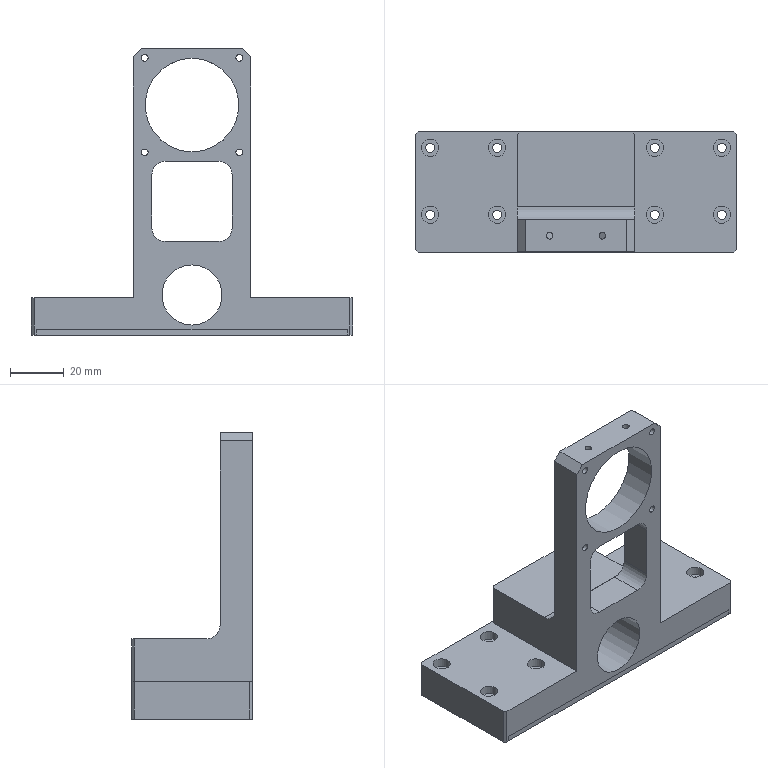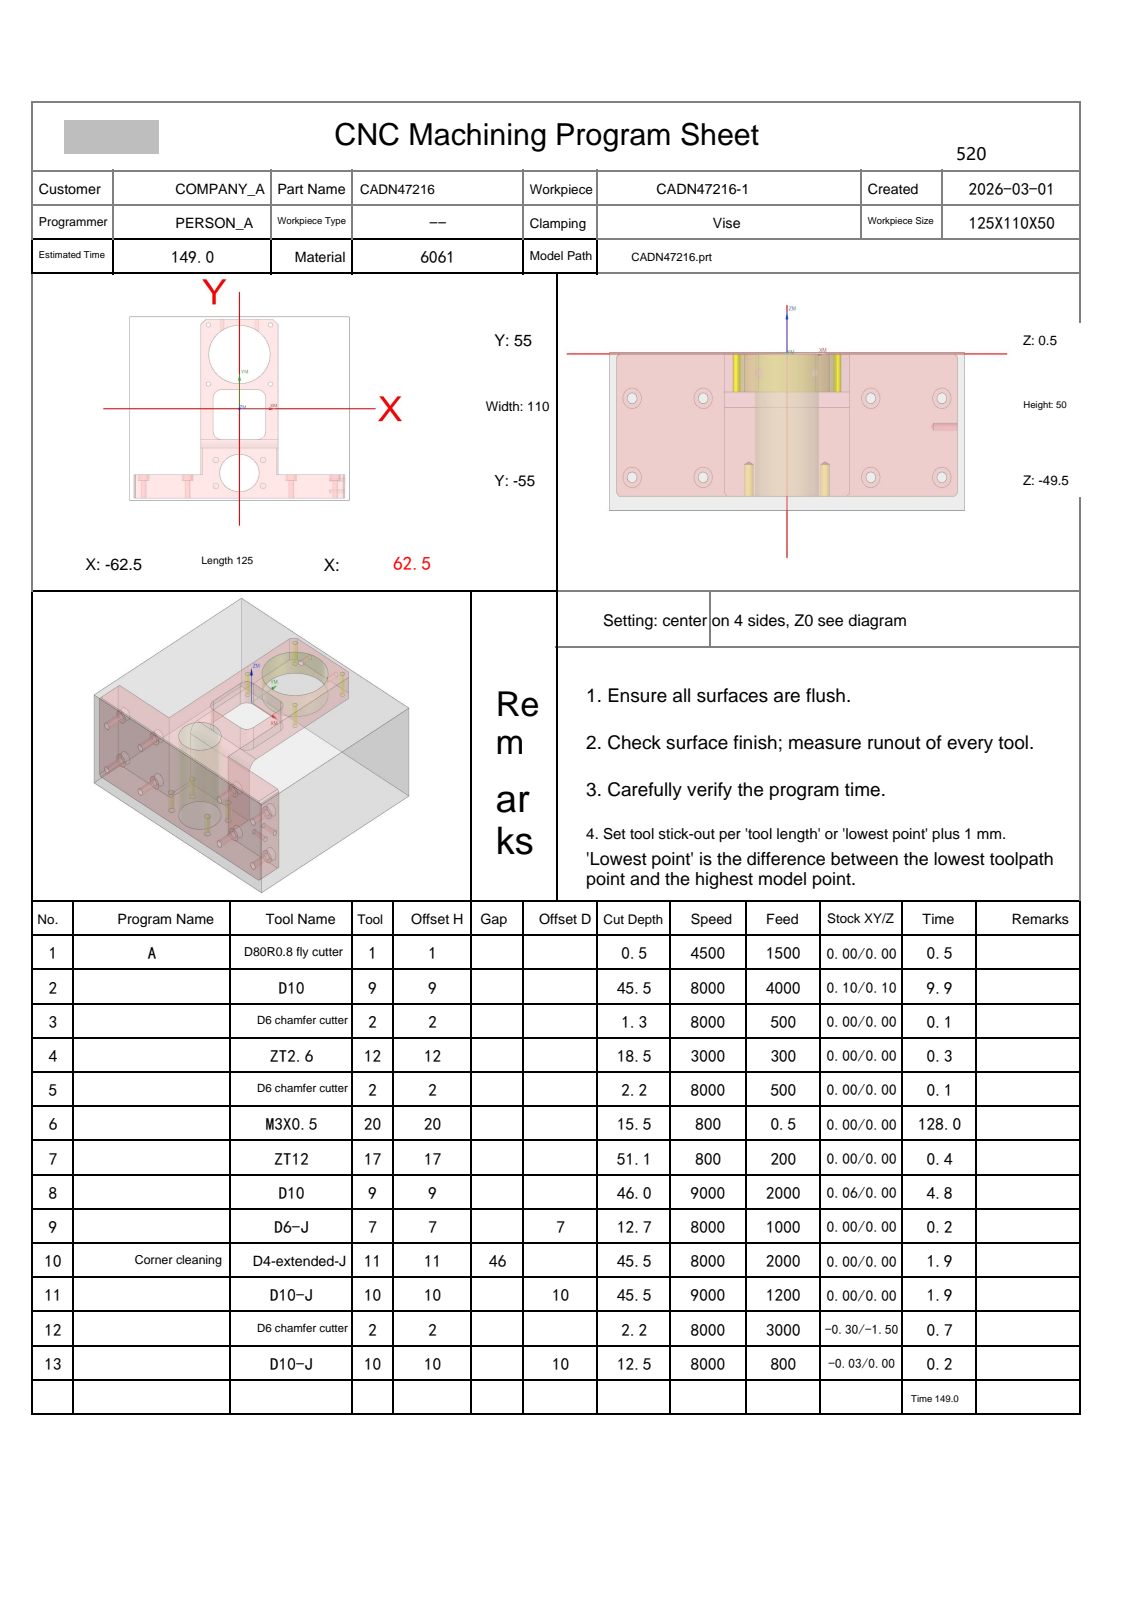NC program | NX | posted by the shop | part box 120 x 45 x 107 mm
Lines 6042 to 6508 of 16292:
N3 T02 M06
(D6 chamfer cutter  D=6. R=0. H=02 ce=0.00 di=0.10)
G00 G90 G54 X-17.678 Y50.178 M03 S8000
G43 H02 Z50.
M08
G98 G81 X-17.678 Y50.178 Z-.8 R1. F500.
X17.678
Y14.822
X0.0 Y32.5
X-17.678 Y14.822
X0.0 Y-38.5
G80
G00 Z50.
G91 G28 Z0.0
M05
M09
G91 G28 Z0.0
M01
N4 T12 M06
(ZT2.6 D=2.6 DR_a=118 H=12)
G00 G90 G54 X-17.678 Y50.178 M03 S3000
G43 H12 Z50.
M08
G98 G83 X-17.678 Y50.178 Z-18. R1. F300. Q2.
Y14.822
X17.678
Y50.178
G80
G00 Z50.
G91 G28 Z0.0
M05
M09
G91 G28 Z0.0
M01
N5 T02 M06
(D6 chamfer cutter  D=6. R=0. H=02 ce=0.00 di=0.10)
G00 G90 G54 X-17.678 Y50.178 M03 S8000
G43 H02 Z50.
M08
G98 G81 X-17.678 Y50.178 Z-1.75 R3. F500.
Y14.822
X17.678
Y50.178
G80
G00 Z50.
G91 G28 Z0.0
M05
M09
G91 G28 Z0.0
M01
N6 T20 M06
(M3X0.5 D=2.5 DR_a=180 H=20)
G00 G90 G54 X-17.678 Y50.178 M03 S800
G43 H20 Z50.
M08
G95
G98 G84 X-17.678 Y50.178 Z-15. R1. F.5 Q5.
Y14.822
X17.678
Y50.178
G80
G94
G00 Z50.
G91 G28 Z0.0
M05
M09
G91 G28 Z0.0
M01
N7 T17 M06
(ZT12 D=12. DR_a=118 H=17)
G00 G90 G54 X0.0 Y-38.5 M03 S800
G43 H17 Z50.
M08
G98 G83 X0.0 Y-38.5 Z-50.605 R1. F200. Q3.
G80
G00 Z50.
G00 G90 X0.0 Y32.5 M03 S800
Z50.
G98 G83 X0.0 Y32.5 Z-17.105 R1. F200. Q2.
G80
G00 Z50.
G91 G28 Z0.0
M05
M09
G91 G28 Z0.0
M01
N8 T09 M06
(D10  D=10. R=0. H=09 ce=0.10 di=0.00)
G00 G90 G54 X0.0 Y-13.4 M03 S9000
G43 H09 Z50.
M08
Z.5
G01 X9.9 Z.44 F2000.
Y6.4 Z.319
X-9.9 Z.199
Y-13.4 Z.079
X9.9 Z-.042
Y6.4 Z-.162
X-9.9 Z-.282
Y-13.4 Z-.403
X9.9 Z-.523
Y6.4 Z-.644
X-9.9 Z-.764
Y-13.4 Z-.884
X9.9 Z-1.005
Y6.4 Z-1.125
X-9.9 Z-1.245
Y-13.4 Z-1.366
X9.9 Z-1.486
Y6.4 Z-1.606
X-9.9 Z-1.727
Y-13.4 Z-1.847
X9.9 Z-1.968
Y6.4 Z-2.088
X-9.9 Z-2.208
Y-13.4 Z-2.329
X9.9 Z-2.449
Y6.4 Z-2.569
X-9.9 Z-2.69
Y-13.4 Z-2.81
X9.9 Z-2.931
Y6.4 Z-3.051
X-9.9 Z-3.171
Y-13.4 Z-3.292
X9.9 Z-3.412
Y6.4 Z-3.532
X-9.9 Z-3.653
Y-13.4 Z-3.773
X9.9 Z-3.894
Y6.4 Z-4.014
X-9.9 Z-4.134
Y-13.4 Z-4.255
X9.9 Z-4.375
Y6.4 Z-4.495
X-9.9 Z-4.616
Y-13.4 Z-4.736
X9.9 Z-4.856
Y6.4 Z-4.977
X-9.9 Z-5.097
Y-13.4 Z-5.218
X9.9 Z-5.338
Y6.4 Z-5.458
X-9.9 Z-5.579
Y-13.4 Z-5.699
X9.9 Z-5.819
Y6.4 Z-5.94
X-9.9 Z-6.06
Y-13.4 Z-6.181
X9.9 Z-6.301
Y6.4 Z-6.421
X-9.9 Z-6.542
Y-13.4 Z-6.662
X9.9 Z-6.782
Y6.4 Z-6.903
X-9.9 Z-7.023
Y-13.4 Z-7.144
X9.9 Z-7.264
Y6.4 Z-7.384
X-9.9 Z-7.505
Y-13.4 Z-7.625
X9.9 Z-7.745
Y6.4 Z-7.866
X-9.9 Z-7.986
Y-13.4 Z-8.106
X9.9 Z-8.227
Y6.4 Z-8.347
X-9.9 Z-8.468
Y-13.4 Z-8.588
X9.9 Z-8.708
Y6.4 Z-8.829
X-9.9 Z-8.949
Y-13.4 Z-9.069
X9.9 Z-9.19
Y6.4 Z-9.31
X-9.9 Z-9.431
Y-13.4 Z-9.551
X9.9 Z-9.671
Y6.4 Z-9.792
X-9.9 Z-9.912
Y-13.4 Z-10.032
X9.9 Z-10.153
Y6.4 Z-10.273
X-9.9 Z-10.394
Y-13.4 Z-10.514
X9.9 Z-10.634
Y6.4 Z-10.755
X-9.9 Z-10.875
Y-13.4 Z-10.995
X9.9 Z-11.116
Y6.4 Z-11.236
X-9.9 Z-11.356
Y-13.4 Z-11.477
X9.9 Z-11.597
Y6.4 Z-11.718
X-9.9 Z-11.838
Y-13.4 Z-11.958
X9.9 Z-12.079
Y6.4 Z-12.199
X-9.9 Z-12.319
Y-13.4 Z-12.44
X0.0 Z-12.5
X9.9
Y6.4
X-9.9
Y-13.4
X0.0
X.5
Z-11.5
G00 Z50.
G00 G90 X0.0 Y-38.5 M03 S8000
Z50.
Z.5
G03 X3.075 Y-41.575 I3.075 J0.0 F2000.
X6.15 Y-38.5 I0.0 J3.075
X6.15 Y-38.5 Z0.0 I-6.15 J0.0
X6.15 Y-38.5 Z-.5 I-6.15 J0.0
X6.15 Y-38.5 Z-1. I-6.15 J0.0
X6.15 Y-38.5 Z-1.5 I-6.15 J0.0
X6.15 Y-38.5 Z-2. I-6.15 J0.0
X6.15 Y-38.5 Z-2.5 I-6.15 J0.0
X6.15 Y-38.5 Z-3. I-6.15 J0.0
X6.15 Y-38.5 Z-3.5 I-6.15 J0.0
X6.15 Y-38.5 Z-4. I-6.15 J0.0
X6.15 Y-38.5 Z-4.5 I-6.15 J0.0
X6.15 Y-38.5 Z-5. I-6.15 J0.0
X6.15 Y-38.5 Z-5.5 I-6.15 J0.0
X6.15 Y-38.5 Z-6. I-6.15 J0.0
X6.15 Y-38.5 Z-6.5 I-6.15 J0.0
X6.15 Y-38.5 Z-7. I-6.15 J0.0
X6.15 Y-38.5 Z-7.5 I-6.15 J0.0
X6.15 Y-38.5 Z-8. I-6.15 J0.0
X6.15 Y-38.5 Z-8.5 I-6.15 J0.0
X6.15 Y-38.5 Z-9. I-6.15 J0.0
X6.15 Y-38.5 Z-9.5 I-6.15 J0.0
X6.15 Y-38.5 Z-10. I-6.15 J0.0
X6.15 Y-38.5 Z-10.5 I-6.15 J0.0
X6.15 Y-38.5 Z-11. I-6.15 J0.0
X6.15 Y-38.5 Z-11.5 I-6.15 J0.0
X6.15 Y-38.5 Z-12. I-6.15 J0.0
X6.15 Y-38.5 Z-12.5 I-6.15 J0.0
X6.15 Y-38.5 Z-13. I-6.15 J0.0
X6.15 Y-38.5 Z-13.5 I-6.15 J0.0
X6.15 Y-38.5 Z-14. I-6.15 J0.0
X6.15 Y-38.5 Z-14.5 I-6.15 J0.0
X6.15 Y-38.5 Z-15. I-6.15 J0.0
X6.15 Y-38.5 Z-15.5 I-6.15 J0.0
X6.15 Y-38.5 Z-16. I-6.15 J0.0
X6.15 Y-38.5 Z-16.5 I-6.15 J0.0
X6.15 Y-38.5 Z-17. I-6.15 J0.0
X6.15 Y-38.5 Z-17.5 I-6.15 J0.0
X6.15 Y-38.5 Z-18. I-6.15 J0.0
X6.15 Y-38.5 Z-18.5 I-6.15 J0.0
X6.15 Y-38.5 Z-19. I-6.15 J0.0
X6.15 Y-38.5 Z-19.5 I-6.15 J0.0
X6.15 Y-38.5 Z-20. I-6.15 J0.0
X6.15 Y-38.5 Z-20.5 I-6.15 J0.0
X6.15 Y-38.5 Z-21. I-6.15 J0.0
X6.15 Y-38.5 Z-21.5 I-6.15 J0.0
X6.15 Y-38.5 Z-22. I-6.15 J0.0
X6.15 Y-38.5 Z-22.5 I-6.15 J0.0
X6.15 Y-38.5 Z-23. I-6.15 J0.0
X6.15 Y-38.5 Z-23.5 I-6.15 J0.0
X6.15 Y-38.5 Z-24. I-6.15 J0.0
X6.15 Y-38.5 Z-24.5 I-6.15 J0.0
X6.15 Y-38.5 Z-25. I-6.15 J0.0
X6.15 Y-38.5 Z-25.5 I-6.15 J0.0
X6.15 Y-38.5 Z-26. I-6.15 J0.0
X6.15 Y-38.5 Z-26.5 I-6.15 J0.0
X6.15 Y-38.5 Z-27. I-6.15 J0.0
X6.15 Y-38.5 Z-27.5 I-6.15 J0.0
X6.15 Y-38.5 Z-28. I-6.15 J0.0
X6.15 Y-38.5 Z-28.5 I-6.15 J0.0
X6.15 Y-38.5 Z-29. I-6.15 J0.0
X6.15 Y-38.5 Z-29.5 I-6.15 J0.0
X6.15 Y-38.5 Z-30. I-6.15 J0.0
X6.15 Y-38.5 Z-30.5 I-6.15 J0.0
X6.15 Y-38.5 Z-31. I-6.15 J0.0
X6.15 Y-38.5 Z-31.5 I-6.15 J0.0
X6.15 Y-38.5 Z-32. I-6.15 J0.0
X6.15 Y-38.5 Z-32.5 I-6.15 J0.0
X6.15 Y-38.5 Z-33. I-6.15 J0.0
X6.15 Y-38.5 Z-33.5 I-6.15 J0.0
X6.15 Y-38.5 Z-34. I-6.15 J0.0
X6.15 Y-38.5 Z-34.5 I-6.15 J0.0
X6.15 Y-38.5 Z-35. I-6.15 J0.0
X6.15 Y-38.5 Z-35.5 I-6.15 J0.0
X6.15 Y-38.5 Z-36. I-6.15 J0.0
X6.15 Y-38.5 Z-36.5 I-6.15 J0.0
X6.15 Y-38.5 Z-37. I-6.15 J0.0
X6.15 Y-38.5 Z-37.5 I-6.15 J0.0
X6.15 Y-38.5 Z-38. I-6.15 J0.0
X6.15 Y-38.5 Z-38.5 I-6.15 J0.0
X6.15 Y-38.5 Z-39. I-6.15 J0.0
X6.15 Y-38.5 Z-39.5 I-6.15 J0.0
X6.15 Y-38.5 Z-40. I-6.15 J0.0
X6.15 Y-38.5 Z-40.5 I-6.15 J0.0
X6.15 Y-38.5 Z-41. I-6.15 J0.0
X6.15 Y-38.5 Z-41.5 I-6.15 J0.0
X6.15 Y-38.5 Z-42. I-6.15 J0.0
X6.15 Y-38.5 Z-42.5 I-6.15 J0.0
X6.15 Y-38.5 Z-43. I-6.15 J0.0
X6.15 Y-38.5 Z-43.5 I-6.15 J0.0
X6.15 Y-38.5 Z-44. I-6.15 J0.0
X6.15 Y-38.5 Z-44.5 I-6.15 J0.0
X6.15 Y-38.5 Z-45. I-6.15 J0.0
X6.15 Y-38.5 Z-45.5 I-6.15 J0.0
X0.0 Y-32.35 I-6.15 J0.0
X-6.15 Y-38.5 I0.0 J-6.15
X0.0 Y-44.65 I6.15 J0.0
X6.15 Y-38.5 I0.0 J6.15
X3.075 Y-35.425 I-3.075 J0.0
X0.0 Y-38.5 I0.0 J-3.075
G00 Z50.
G00 G90 X0.0 Y32.5 M03 S8000
Z50.
Z.5
G03 X2.073 Y30.427 I2.073 J0.0 F2000.
X4.147 Y32.5 I0.0 J2.073
X4.147 Y32.5 Z-.1 I-4.147 J0.0
X4.147 Y32.5 Z-.7 I-4.147 J0.0
X4.147 Y32.5 Z-1.3 I-4.147 J0.0
X4.147 Y32.5 Z-1.9 I-4.147 J0.0
X4.147 Y32.5 Z-2.5 I-4.147 J0.0
X4.147 Y32.5 Z-3.1 I-4.147 J0.0
X4.147 Y32.5 Z-3.7 I-4.147 J0.0
X4.147 Y32.5 Z-4.3 I-4.147 J0.0
X4.147 Y32.5 Z-4.9 I-4.147 J0.0
X4.147 Y32.5 Z-5.5 I-4.147 J0.0
X4.147 Y32.5 Z-6.1 I-4.147 J0.0
X4.147 Y32.5 Z-6.7 I-4.147 J0.0
X4.147 Y32.5 Z-7.3 I-4.147 J0.0
X4.147 Y32.5 Z-7.9 I-4.147 J0.0
X4.147 Y32.5 Z-8.5 I-4.147 J0.0
X4.147 Y32.5 Z-9.1 I-4.147 J0.0
X4.147 Y32.5 Z-9.7 I-4.147 J0.0
X4.147 Y32.5 Z-10.3 I-4.147 J0.0
X4.147 Y32.5 Z-10.9 I-4.147 J0.0
X4.147 Y32.5 Z-11.5 I-4.147 J0.0
X4.147 Y32.5 Z-12.1 I-4.147 J0.0
X-2.073 Y28.909 Z-12.5 I-4.147 J0.0
X0.0 Y28.353 I2.073 J3.591
X4.147 Y32.5 I0.0 J4.147
X0.0 Y36.647 I-4.147 J0.0
X-4.147 Y32.5 I0.0 J-4.147
X-2.073 Y28.909 I4.147 J0.0
X-1.037 Y28.631 I1.037 J1.796
X1.037 Y30.704 I0.0 J2.073
X0.0 Y32.5 I-2.073 J0.0
G00 Z.5
G03 X4.147 Y28.353 I4.147 J0.0
X8.293 Y32.5 I0.0 J4.147
X8.293 Y32.5 Z-.1 I-8.293 J0.0
X8.293 Y32.5 Z-.7 I-8.293 J0.0
X8.293 Y32.5 Z-1.3 I-8.293 J0.0
X8.293 Y32.5 Z-1.9 I-8.293 J0.0
X8.293 Y32.5 Z-2.5 I-8.293 J0.0
X8.293 Y32.5 Z-3.1 I-8.293 J0.0
X8.293 Y32.5 Z-3.7 I-8.293 J0.0
X8.293 Y32.5 Z-4.3 I-8.293 J0.0
X8.293 Y32.5 Z-4.9 I-8.293 J0.0
X8.293 Y32.5 Z-5.5 I-8.293 J0.0
X8.293 Y32.5 Z-6.1 I-8.293 J0.0
X8.293 Y32.5 Z-6.7 I-8.293 J0.0
X8.293 Y32.5 Z-7.3 I-8.293 J0.0
X8.293 Y32.5 Z-7.9 I-8.293 J0.0
X8.293 Y32.5 Z-8.5 I-8.293 J0.0
X8.293 Y32.5 Z-9.1 I-8.293 J0.0
X8.293 Y32.5 Z-9.7 I-8.293 J0.0
X8.293 Y32.5 Z-10.3 I-8.293 J0.0
X8.293 Y32.5 Z-10.9 I-8.293 J0.0
X8.293 Y32.5 Z-11.5 I-8.293 J0.0
X8.293 Y32.5 Z-12.1 I-8.293 J0.0
X-4.147 Y25.318 Z-12.5 I-8.293 J0.0
X0.0 Y24.207 I4.147 J7.182
X8.293 Y32.5 I0.0 J8.293
X0.0 Y40.793 I-8.293 J0.0
X-8.293 Y32.5 I0.0 J-8.293
X-4.147 Y25.318 I8.293 J0.0
X-2.073 Y24.762 I2.073 J3.591
X2.073 Y28.909 I0.0 J4.147
X0.0 Y32.5 I-4.147 J0.0
G00 Z.5
G03 X6.22 Y26.28 I6.22 J0.0
X12.44 Y32.5 I0.0 J6.22
X12.44 Y32.5 Z-.1 I-12.44 J0.0
X12.44 Y32.5 Z-.7 I-12.44 J0.0
X12.44 Y32.5 Z-1.3 I-12.44 J0.0
X12.44 Y32.5 Z-1.9 I-12.44 J0.0
X12.44 Y32.5 Z-2.5 I-12.44 J0.0
X12.44 Y32.5 Z-3.1 I-12.44 J0.0
X12.44 Y32.5 Z-3.7 I-12.44 J0.0
X12.44 Y32.5 Z-4.3 I-12.44 J0.0
X12.44 Y32.5 Z-4.9 I-12.44 J0.0
X12.44 Y32.5 Z-5.5 I-12.44 J0.0
X12.44 Y32.5 Z-6.1 I-12.44 J0.0
X12.44 Y32.5 Z-6.7 I-12.44 J0.0
X12.44 Y32.5 Z-7.3 I-12.44 J0.0
X12.44 Y32.5 Z-7.9 I-12.44 J0.0
X12.44 Y32.5 Z-8.5 I-12.44 J0.0
X12.44 Y32.5 Z-9.1 I-12.44 J0.0
X12.44 Y32.5 Z-9.7 I-12.44 J0.0
X12.44 Y32.5 Z-10.3 I-12.44 J0.0
X12.44 Y32.5 Z-10.9 I-12.44 J0.0
X12.44 Y32.5 Z-11.5 I-12.44 J0.0
X12.44 Y32.5 Z-12.1 I-12.44 J0.0
X-6.22 Y21.727 Z-12.5 I-12.44 J0.0
X0.0 Y20.06 I6.22 J10.773
X12.44 Y32.5 I0.0 J12.44
X0.0 Y44.94 I-12.44 J0.0
X-12.44 Y32.5 I0.0 J-12.44
X-6.22 Y21.727 I12.44 J0.0
X-3.11 Y20.893 I3.11 J5.387
X3.11 Y27.113 I0.0 J6.22
X0.0 Y32.5 I-6.22 J0.0
G00 Z50.
G91 G28 Z0.0
M05
M09
G91 G28 Z0.0
M01
N9 T07 M06
(D6-J  D=6. R=0. H=07 ce=0.00 di=0.00)
G00 G90 G54 X-10.707 Y-14.207 M03 S8000
G43 H07 Z50.
M08
Z-5.6
G01 Z-6.1 F1000.
G41 D07
X-11. Y-14.5
G03 X-10. Y-15.5 I1. J0.0
G01 X10.
G03 X12. Y-13.5 I0.0 J2.
G01 Y6.5
G03 X10. Y8.5 I-2. J0.0
G01 X-10.
G03 X-12. Y6.5 I0.0 J-2.
G01 Y-13.5
G03 X-10. Y-15.5 I2. J0.0
G01 X-9.5
G03 X-8.5 Y-14.5 I0.0 J1.
G01 G40 Y-14.4
Z-5.6
G00 Z50.
X-10.707 Y-14.207
Z-11.7
G01 Z-12.2
G41 D07
X-11. Y-14.5
G03 X-10. Y-15.5 I1. J0.0
G01 X10.
G03 X12. Y-13.5 I0.0 J2.
G01 Y6.5
G03 X10. Y8.5 I-2. J0.0
G01 X-10.
G03 X-12. Y6.5 I0.0 J-2.
G01 Y-13.5
G03 X-10. Y-15.5 I2. J0.0
G01 X-9.5
G03 X-8.5 Y-14.5 I0.0 J1.
G01 G40 Y-14.4
Z-11.7
G00 Z50.
G91 G28 Z0.0
M05
M09
G91 G28 Z0.0
M01